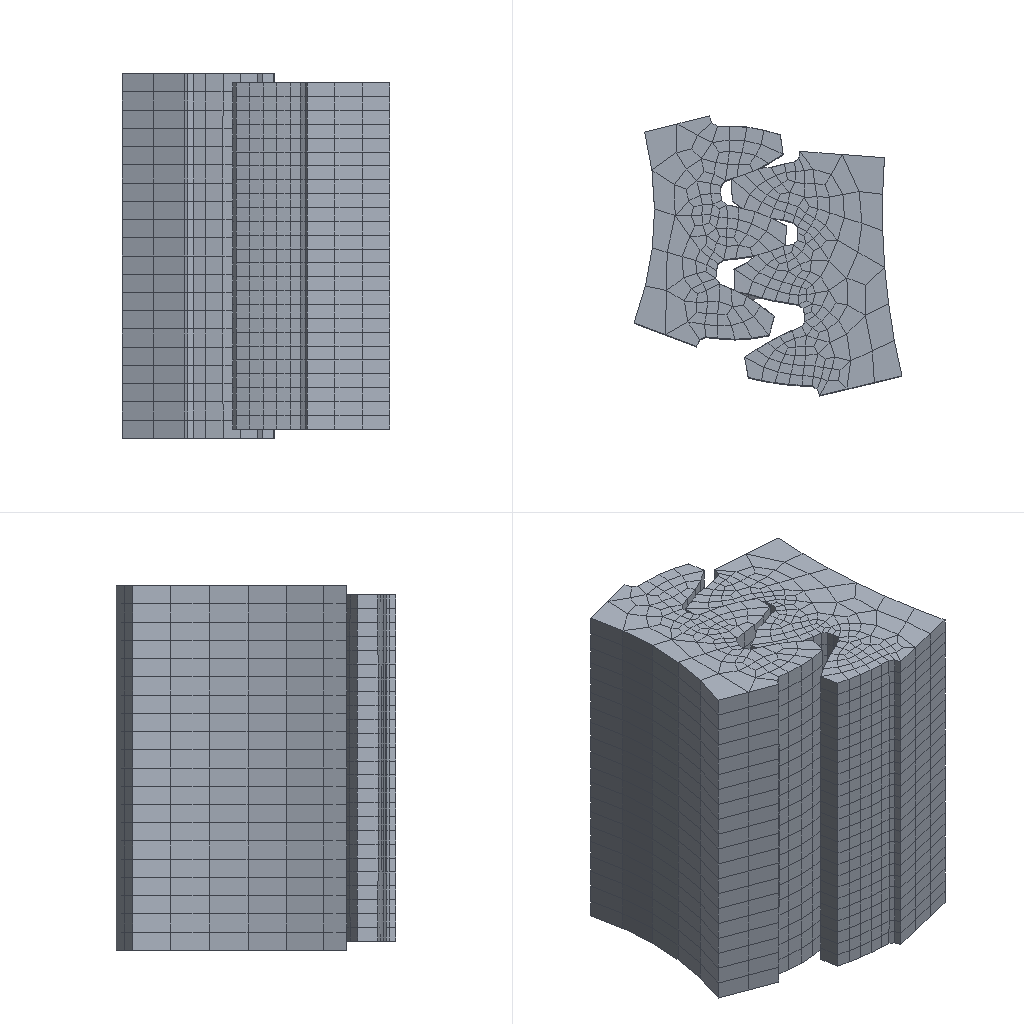Simulation study | abaqus
Set-up summary:
category,name,step,type,value,unit,region
solver,abaqus
solver,version,,,Abaqus/Standard 3DEXPERIENCE R2017x
units,not stated in the deck,,not stated
analysis,deck,,static,static
load_step,Step-1,Step-1,static
load_step,requested,,,1
mesh,nodes,,,7822
mesh,elements,,,6270
element_type,C3D8,,solid,6270
load,load commands in deck,,count,1
bc,support commands in deck,,count,10
material,MATERIAL-1,,in results
check,setup vs results,,match,"per instance, exact: element labels, types and connectivity; labels of the nodes the elements use; coordinates of those nodes at SINGLE_PRECISION in 1 of 2 instance(s)"
Abaqus input file, long lists of numbers shortened:
*Heading
** Job name: Job-1 Model name: Model-1
** Generated by: Abaqus/CAE 2017
*Preprint, echo=NO, model=NO, history=NO, contact=NO
**
** PARTS
**
*Part, name=work-1
*Node
      1,   53.087,  -20.275,         -39.
      2,   62.131,   -18.116,         -39.
** (4964 more lines like these left out)
*Element, type=C3D8
   1,  169,  189,  126,  144,  360,  380,  317,  335
   2,    9,   10,  100,   60,  200,  201,  291,  251
** (4048 more lines like these left out)
*Nset, nset=Set-6, generate
    1,  4966,     1
*Elset, elset=Set-6, generate
    1,  4050,     1
** Section: Section-1
*Solid Section, elset=Set-6, material=Material-1
,
*End Part
**
*Part, name=work-2
*Node
      1,   41.,   10.406,         -40.
      2,   33.924,    8.61,         -40.
** (2854 more lines like these left out)
*Element, type=C3D8
   1,   98,  101,   83,  111,  234,  237,  219,  247
   2,    6,   76,   60,    5,  142,  212,  196,  141
** (2218 more lines like these left out)
*Nset, nset=Set-5, generate
    1,  2856,     1
*Elset, elset=Set-5, generate
    1,  2220,     1
** Section: Section-1
*Solid Section, elset=Set-5, material=Material-1
,
*End Part
**
**
** ASSEMBLY
**
*Assembly, name=Assembly
**
*Instance, name=work-1-1, part=work-1
*End Instance
**
*Instance, name=work-2-1, part=work-2
*End Instance
**
*Node
      1,  -2.55795385e-13,  -3.55271368e-15,         -20.
*Node
      2,         138.,  -1.33226763e-15,         -20.
*Nset, nset=Set-3
 2,
*Nset, nset=Set-4
 1,
*Nset, nset=Set-6, instance=work-1-1, generate
    1,  4966,     1
*Nset, nset=Set-6, instance=work-2-1, generate
    1,  2856,     1
*Elset, elset=Set-6, instance=work-1-1, generate
    1,  4050,     1
*Elset, elset=Set-6, instance=work-2-1, generate
    1,  2220,     1
*Nset, nset=Set-7
 1,
*Nset, nset=Set-8, instance=work-1-1, generate
    1,  4966,     1
*Nset, nset=Set-8, instance=work-2-1, generate
    1,  2856,     1
*Elset, elset=Set-8, instance=work-1-1, generate
    1,  4050,     1
*Elset, elset=Set-8, instance=work-2-1, generate
    1,  2220,     1
*Nset, nset=m_Set-1
 1,
*Nset, nset=m_Set-2
 2,
*Nset, nset=_PickedSet18, internal, instance=work-1-1, generate
    1,  4966,     1
*Nset, nset=_PickedSet18, internal, instance=work-2-1, generate
    1,  2856,     1
*Elset, elset=_PickedSet18, internal, instance=work-1-1, generate
    1,  4050,     1
*Elset, elset=_PickedSet18, internal, instance=work-2-1, generate
    1,  2220,     1
*Elset, elset=_m_Surf-3_S6, internal, instance=work-2-1
    2,   13,   15,   16,   19,   22,   24,   25,   29,   31,   32,   33,   35,  113,  124,  126
  127,  130,  133,  135,  136,  140,  142,  143,  144,  146,  224,  235,  237,  238,  241,  244
** (15 more lines like these left out)
*Elset, elset=_m_Surf-3_S5, internal, instance=work-2-1
   38,   46,  149,  157,  260,  268,  371,  379,  482,  490,  593,  601,  704,  712,  815,  823
  926,  934, 1037, 1045, 1148, 1156, 1259, 1267, 1370, 1378, 1481, 1489, 1592, 1600, 1703, 1711
** (1 more lines like these left out)
*Elset, elset=_m_Surf-3_S4, internal, instance=work-2-1
    5,    6,   11,   12,   27,   45,   48,   49,   54,   57,   59,   60,   62,   79,   80,   81
  116,  117,  122,  123,  138,  156,  159,  160,  165,  168,  170,  171,  173,  190,  191,  192
** (18 more lines like these left out)
*Elset, elset=_m_Surf-3_S3, internal, instance=work-2-1
    4,    9,   10,   20,   28,   59,   60,   62,  115,  120,  121,  131,  139,  170,  171,  173
  226,  231,  232,  242,  250,  281,  282,  284,  337,  342,  343,  353,  361,  392,  393,  395
** (8 more lines like these left out)
*Surface, type=ELEMENT, name=m_Surf-3
_m_Surf-3_S6, S6
_m_Surf-3_S5, S5
_m_Surf-3_S4, S4
_m_Surf-3_S3, S3
*Elset, elset=_s_Surf-1_S6, internal, instance=work-2-1, generate
   37,  2146,   111
*Elset, elset=_s_Surf-1_S3, internal, instance=work-2-1
   42,   93,  153,  204,  264,  315,  375,  426,  486,  537,  597,  648,  708,  759,  819,  870
  930,  981, 1041, 1092, 1152, 1203, 1263, 1314, 1374, 1425, 1485, 1536, 1596, 1647, 1707, 1758
** (1 more lines like these left out)
*Elset, elset=_s_Surf-1_S5, internal, instance=work-2-1
   72,   95,  183,  206,  294,  317,  405,  428,  516,  539,  627,  650,  738,  761,  849,  872
  960,  983, 1071, 1094, 1182, 1205, 1293, 1316, 1404, 1427, 1515, 1538, 1626, 1649, 1737, 1760
** (1 more lines like these left out)
*Surface, type=ELEMENT, name=s_Surf-1
_s_Surf-1_S6, S6
_s_Surf-1_S3, S3
_s_Surf-1_S5, S5
*Elset, elset=_s_Surf-2_S6, internal, instance=work-1-1
   36,  147,  198,  309,  360,  471,  522,  633,  684,  795,  846,  957, 1008, 1119, 1170, 1281
 1332, 1443, 1494, 1605, 1656, 1767, 1818, 1929, 1980, 2091, 2142, 2253, 2304, 2415, 2466, 2577
** (2 more lines like these left out)
*Elset, elset=_s_Surf-2_S5, internal, instance=work-1-1
   51,  145,  213,  307,  375,  469,  537,  631,  699,  793,  861,  955, 1023, 1117, 1185, 1279
 1347, 1441, 1509, 1603, 1671, 1765, 1833, 1927, 1995, 2089, 2157, 2251, 2319, 2413, 2481, 2575
** (2 more lines like these left out)
*Elset, elset=_s_Surf-2_S4, internal, instance=work-1-1, generate
  149,  4037,   162
*Elset, elset=_s_Surf-2_S3, internal, instance=work-1-1, generate
  152,  4040,   162
*Surface, type=ELEMENT, name=s_Surf-2
_s_Surf-2_S6, S6
_s_Surf-2_S5, S5
_s_Surf-2_S4, S4
_s_Surf-2_S3, S3
*Elset, elset=_s_Surf-3_S4, internal, instance=work-1-1
    6,    8,   10,   13,   14,   18,   23,   29,   30,   32,   37,   42,   50,   62,   67,   70
   72,   73,   75,   79,   81,   84,  168,  170,  172,  175,  176,  180,  185,  191,  192,  194
** (33 more lines like these left out)
*Elset, elset=_s_Surf-3_S6, internal, instance=work-1-1
    4,   20,   27,   28,   39,   40,   41,   43,   44,   45,   47,   48,   64,   74,  166,  182
  189,  190,  201,  202,  203,  205,  206,  207,  209,  210,  226,  236,  328,  344,  351,  352
** (20 more lines like these left out)
*Elset, elset=_s_Surf-3_S5, internal, instance=work-1-1
   39,   43,   47,   57,   69,  201,  205,  209,  219,  231,  363,  367,  371,  381,  393,  525
  529,  533,  543,  555,  687,  691,  695,  705,  717,  849,  853,  857,  867,  879, 1011, 1015
** (6 more lines like these left out)
*Elset, elset=_s_Surf-3_S3, internal, instance=work-1-1
    2,   11,   22,   31,  164,  173,  184,  193,  326,  335,  346,  355,  488,  497,  508,  517
  650,  659,  670,  679,  812,  821,  832,  841,  974,  983,  994, 1003, 1136, 1145, 1156, 1165
** (5 more lines like these left out)
*Surface, type=ELEMENT, name=s_Surf-3
_s_Surf-3_S4, S4
_s_Surf-3_S6, S6
_s_Surf-3_S5, S5
_s_Surf-3_S3, S3
** Constraint: Constraint-1
*Coupling, constraint name=Constraint-1, ref node=m_Set-1, surface=s_Surf-1
*Kinematic
** Constraint: Constraint-2
*Coupling, constraint name=Constraint-2, ref node=m_Set-2, surface=s_Surf-2
*Kinematic
*End Assembly
*Amplitude, name=Amp-1
             0.,              0.,             10.,              1.
**
** MATERIALS
**
*Material, name=Material-1
*Elastic
210000., 0.33
**
** INTERACTION PROPERTIES
**
*Surface Interaction, name=IntProp-1
1.,
*Friction, slip tolerance=0.005
 0.3,
*Surface Behavior, pressure-overclosure=HARD
**
** INTERACTIONS
**
** Interaction: Int-1
*Contact Pair, interaction=IntProp-1, type=SURFACE TO SURFACE, adjust=0.3
s_Surf-3, m_Surf-3
** ----------------------------------------------------------------
**
** STEP: Step-1
**
*Step, name=Step-1, nlgeom=YES, inc=1000
*Static, direct, stabilize=0.0002, allsdtol=0.05, continue=NO
0.1, 7.,
**
** BOUNDARY CONDITIONS
**
** Name: [REDACTED] : Displacement/rotation angle
*Boundary
Set-3, 1, 1
Set-3, 2, 2
Set-3, 3, 3
Set-3, 4, 4
Set-3, 5, 5
** Name: [REDACTED] : Displacement/rotation angle
*Boundary
Set-4, 1, 1
Set-4, 2, 2
Set-4, 3, 3
Set-4, 4, 4
Set-4, 5, 5
*Adaptive Mesh Controls, name=Ada-1
1., 0.
*Adaptive Mesh, elset=_PickedSet18, controls=Ada-1, frequency=1, mesh sweeps=5, op=NEW
**
** ADAPTIVE MESH CONSTRAINTS
**
** Name: Ada-Cons-1 Type: 位移/转角
*Adaptive Mesh Constraint, user
Set-8
**
** LOADS
**
** Name: Load-1   Type: Moment
*Cload, amplitude=Amp-1
Set-7, 6, -500000.
**
** OUTPUT REQUESTS
**
*Restart, write, frequency=0
**
** FIELD OUTPUT: F-Output-1
**
*Output, field
*Node Output
CF, RF, U, V
*Element Output, directions=YES
E, LE, MISES, MISESMAX, PE, PEEQ, PEMAG, S, STATUS
*Contact Output
CDISP, CSTRESS
**
** HISTORY OUTPUT: H-Output-1
**
*Output, history, variable=PRESELECT
*End Step
Results summary:
result,step,,partial,increments=66 time=6.6/7.0
result,analysis,,,static
result,last_loadstep,,,1
result,primary field,,,U
result,reaction total,,FX,0.002721,model units
result,reaction total,,FY,-143.863,model units
result,reaction total,,FZ,-3.9e-05,model units